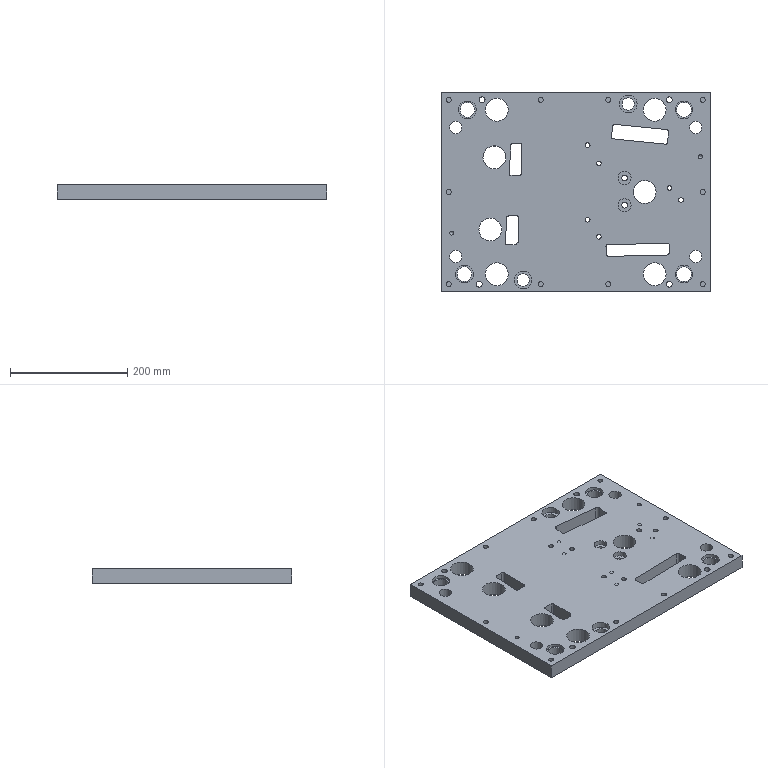Part | NX | features LIN_SOLID_COLOR 2 | 1 solid | 146 faces | box 460 x 340 x 25 mm | volume 3324874 mm3 | cylinder 84 | plane 60 | cone 2 | commonest cylinder face diameters 10 x16 6 x10 8.5 x10 6.8 x8 39 x7 8.001 x6